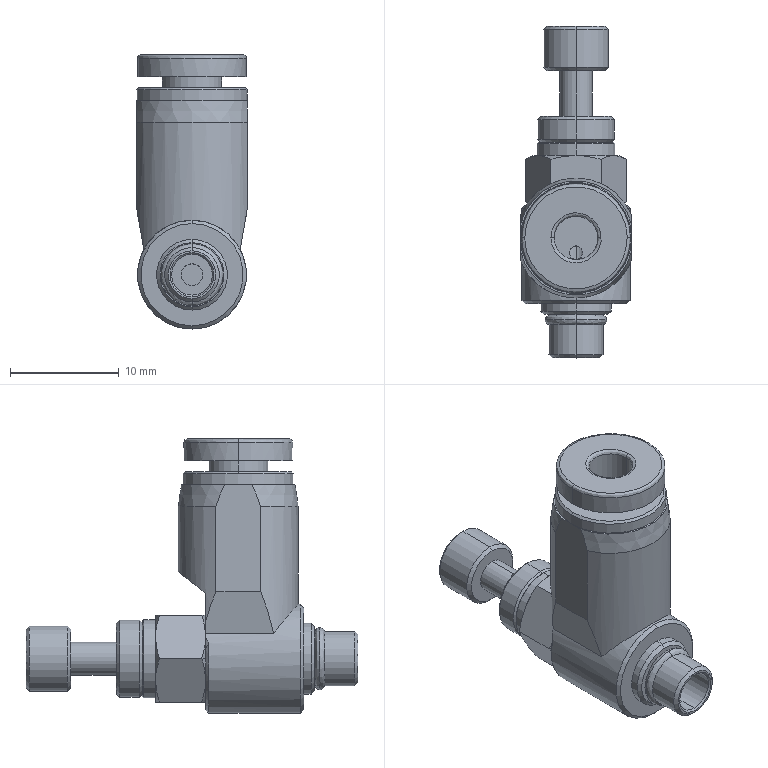Part | STEP file | KZB668-04-M5-668 | 1 solid | 107 faces | box 10.2 x 30.5 x 25.2 mm | volume 2441 mm3 | cone 37 | cylinder 34 | plane 28 | spline 8 | commonest cylinder face diameters 10 x4 11 x4 1.233 x2 2 x2 3 x2 3.75 x2